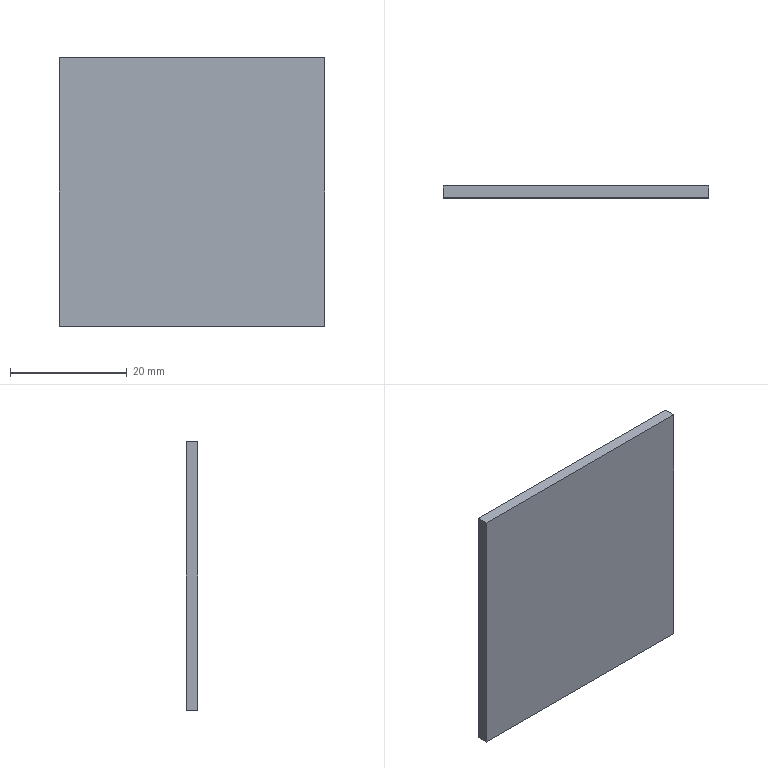Part | Creo | 1 solid | 6 faces | box 45.5 x 2 x 46 mm | volume 4186 mm3 | plane 6
STEP:
#1=CARTESIAN_POINT('',(0.,0.,0.));
#2=DIRECTION('',(0.,0.,1.));
#3=DIRECTION('',(1.,0.,0.));
#4=AXIS2_PLACEMENT_3D('',#1,#2,#3);
#5=CARTESIAN_POINT('',(-63.5,246.,-249.));
#6=VERTEX_POINT('',#5);
#7=CARTESIAN_POINT('',(-18.,246.,-249.));
#8=VERTEX_POINT('',#7);
#9=CARTESIAN_POINT('',(-63.5,246.,-249.));
#10=DIRECTION('',(1.,0.,0.));
#11=VECTOR('',#10,45.5);
#12=LINE('',#9,#11);
#13=EDGE_CURVE('',#6,#8,#12,.T.);
#14=ORIENTED_EDGE('',*,*,#13,.F.);
#15=CARTESIAN_POINT('',(-63.5,248.,-249.));
#16=VERTEX_POINT('',#15);
#17=CARTESIAN_POINT('',(-63.5,248.,-249.));
#18=DIRECTION('',(0.,-1.,0.));
#19=VECTOR('',#18,2.);
#20=LINE('',#17,#19);
#21=EDGE_CURVE('',#16,#6,#20,.T.);
#22=ORIENTED_EDGE('',*,*,#21,.F.);
#23=CARTESIAN_POINT('',(-18.,248.,-249.));
#24=VERTEX_POINT('',#23);
#25=CARTESIAN_POINT('',(-18.,248.,-249.));
#26=DIRECTION('',(-1.,0.,0.));
#27=VECTOR('',#26,45.5);
#28=LINE('',#25,#27);
#29=EDGE_CURVE('',#24,#16,#28,.T.);
#30=ORIENTED_EDGE('',*,*,#29,.F.);
#31=CARTESIAN_POINT('',(-18.,246.,-249.));
#32=DIRECTION('',(0.,1.,0.));
#33=VECTOR('',#32,2.);
#34=LINE('',#31,#33);
#35=EDGE_CURVE('',#8,#24,#34,.T.);
#36=ORIENTED_EDGE('',*,*,#35,.F.);
#37=EDGE_LOOP('',(#14,#22,#30,#36));
#38=FACE_OUTER_BOUND('',#37,.F.);
#39=CARTESIAN_POINT('',(-40.75,247.,-249.));
#40=DIRECTION('',(0.,0.,1.));
#41=DIRECTION('',(1.,0.,0.));
#42=AXIS2_PLACEMENT_3D('',#39,#40,#41);
#43=PLANE('',#42);
#44=ADVANCED_FACE('',(#38),#43,.T.);
#45=CARTESIAN_POINT('',(-18.,246.,-295.));
#46=VERTEX_POINT('',#45);
#47=CARTESIAN_POINT('',(-18.,246.,-249.));
#48=DIRECTION('',(0.,0.,-1.));
#49=VECTOR('',#48,46.);
#50=LINE('',#47,#49);
#51=EDGE_CURVE('',#8,#46,#50,.T.);
#52=ORIENTED_EDGE('',*,*,#51,.T.);
#53=CARTESIAN_POINT('',(-63.5,246.,-295.));
#54=VERTEX_POINT('',#53);
#55=CARTESIAN_POINT('',(-18.,246.,-295.));
#56=DIRECTION('',(-1.,0.,0.));
#57=VECTOR('',#56,45.5);
#58=LINE('',#55,#57);
#59=EDGE_CURVE('',#46,#54,#58,.T.);
#60=ORIENTED_EDGE('',*,*,#59,.T.);
#61=CARTESIAN_POINT('',(-63.5,246.,-249.));
#62=DIRECTION('',(0.,0.,-1.));
#63=VECTOR('',#62,46.);
#64=LINE('',#61,#63);
#65=EDGE_CURVE('',#6,#54,#64,.T.);
#66=ORIENTED_EDGE('',*,*,#65,.F.);
#67=ORIENTED_EDGE('',*,*,#13,.T.);
#68=EDGE_LOOP('',(#52,#60,#66,#67));
#69=FACE_OUTER_BOUND('',#68,.F.);
#70=CARTESIAN_POINT('',(-40.75,246.,-295.));
#71=DIRECTION('',(0.,-1.,0.));
#72=DIRECTION('',(0.,0.,-1.));
#73=AXIS2_PLACEMENT_3D('',#70,#71,#72);
#74=PLANE('',#73);
#75=ADVANCED_FACE('',(#69),#74,.T.);
#76=CARTESIAN_POINT('',(-18.,248.,-295.));
#77=VERTEX_POINT('',#76);
#78=CARTESIAN_POINT('',(-18.,248.,-295.));
#79=DIRECTION('',(0.,-1.,0.));
#80=VECTOR('',#79,2.);
#81=LINE('',#78,#80);
#82=EDGE_CURVE('',#77,#46,#81,.T.);
#83=ORIENTED_EDGE('',*,*,#82,.T.);
#84=ORIENTED_EDGE('',*,*,#51,.F.);
#85=ORIENTED_EDGE('',*,*,#35,.T.);
#86=CARTESIAN_POINT('',(-18.,248.,-249.));
#87=DIRECTION('',(0.,0.,-1.));
#88=VECTOR('',#87,46.);
#89=LINE('',#86,#88);
#90=EDGE_CURVE('',#24,#77,#89,.T.);
#91=ORIENTED_EDGE('',*,*,#90,.T.);
#92=EDGE_LOOP('',(#83,#84,#85,#91));
#93=FACE_OUTER_BOUND('',#92,.F.);
#94=CARTESIAN_POINT('',(-18.,247.,-295.));
#95=DIRECTION('',(1.,0.,0.));
#96=DIRECTION('',(0.,0.,-1.));
#97=AXIS2_PLACEMENT_3D('',#94,#95,#96);
#98=PLANE('',#97);
#99=ADVANCED_FACE('',(#93),#98,.T.);
#100=ORIENTED_EDGE('',*,*,#82,.F.);
#101=CARTESIAN_POINT('',(-63.5,248.,-295.));
#102=VERTEX_POINT('',#101);
#103=CARTESIAN_POINT('',(-63.5,248.,-295.));
#104=DIRECTION('',(1.,0.,0.));
#105=VECTOR('',#104,45.5);
#106=LINE('',#103,#105);
#107=EDGE_CURVE('',#102,#77,#106,.T.);
#108=ORIENTED_EDGE('',*,*,#107,.F.);
#109=CARTESIAN_POINT('',(-63.5,246.,-295.));
#110=DIRECTION('',(0.,1.,0.));
#111=VECTOR('',#110,2.);
#112=LINE('',#109,#111);
#113=EDGE_CURVE('',#54,#102,#112,.T.);
#114=ORIENTED_EDGE('',*,*,#113,.F.);
#115=ORIENTED_EDGE('',*,*,#59,.F.);
#116=EDGE_LOOP('',(#100,#108,#114,#115));
#117=FACE_OUTER_BOUND('',#116,.F.);
#118=CARTESIAN_POINT('',(-40.75,247.,-295.));
#119=DIRECTION('',(0.,0.,-1.));
#120=DIRECTION('',(-1.,0.,0.));
#121=AXIS2_PLACEMENT_3D('',#118,#119,#120);
#122=PLANE('',#121);
#123=ADVANCED_FACE('',(#117),#122,.T.);
#124=CARTESIAN_POINT('',(-63.5,248.,-249.));
#125=DIRECTION('',(0.,0.,-1.));
#126=VECTOR('',#125,46.);
#127=LINE('',#124,#126);
#128=EDGE_CURVE('',#16,#102,#127,.T.);
#129=ORIENTED_EDGE('',*,*,#128,.T.);
#130=ORIENTED_EDGE('',*,*,#107,.T.);
#131=ORIENTED_EDGE('',*,*,#90,.F.);
#132=ORIENTED_EDGE('',*,*,#29,.T.);
#133=EDGE_LOOP('',(#129,#130,#131,#132));
#134=FACE_OUTER_BOUND('',#133,.F.);
#135=CARTESIAN_POINT('',(-40.75,248.,-295.));
#136=DIRECTION('',(0.,1.,0.));
#137=DIRECTION('',(0.,0.,1.));
#138=AXIS2_PLACEMENT_3D('',#135,#136,#137);
#139=PLANE('',#138);
#140=ADVANCED_FACE('',(#134),#139,.T.);
#141=ORIENTED_EDGE('',*,*,#65,.T.);
#142=ORIENTED_EDGE('',*,*,#113,.T.);
#143=ORIENTED_EDGE('',*,*,#128,.F.);
#144=ORIENTED_EDGE('',*,*,#21,.T.);
#145=EDGE_LOOP('',(#141,#142,#143,#144));
#146=FACE_OUTER_BOUND('',#145,.F.);
#147=CARTESIAN_POINT('',(-63.5,247.,-295.));
#148=DIRECTION('',(-1.,0.,0.));
#149=DIRECTION('',(0.,0.,1.));
#150=AXIS2_PLACEMENT_3D('',#147,#148,#149);
#151=PLANE('',#150);
#152=ADVANCED_FACE('',(#146),#151,.T.);
#153=CLOSED_SHELL('',(#44,#75,#99,#123,#140,#152));
#154=MANIFOLD_SOLID_BREP('',#153);
#155=(LENGTH_UNIT()NAMED_UNIT(*)SI_UNIT(.MILLI.,.METRE.));
#156=UNCERTAINTY_MEASURE_WITH_UNIT(LENGTH_MEASURE(0.006473),#155,'','');
#157=(NAMED_UNIT(*)PLANE_ANGLE_UNIT()SI_UNIT($,.RADIAN.));
#158=PLANE_ANGLE_MEASURE_WITH_UNIT(PLANE_ANGLE_MEASURE(0.01745),#157);
#159=(CONVERSION_BASED_UNIT('DEGREE',#158)NAMED_UNIT(*)PLANE_ANGLE_UNIT());
#160=(NAMED_UNIT(*)SI_UNIT($,.STERADIAN.)SOLID_ANGLE_UNIT());
#161=(GEOMETRIC_REPRESENTATION_CONTEXT(3)GLOBAL_UNCERTAINTY_ASSIGNED_CONTEXT((#156))GLOBAL_UNIT_ASSIGNED_CONTEXT((#155,#159,#160))REPRESENTATION_CONTEXT('',''));
#162=ADVANCED_BREP_SHAPE_REPRESENTATION('',(#4,#154),#161);